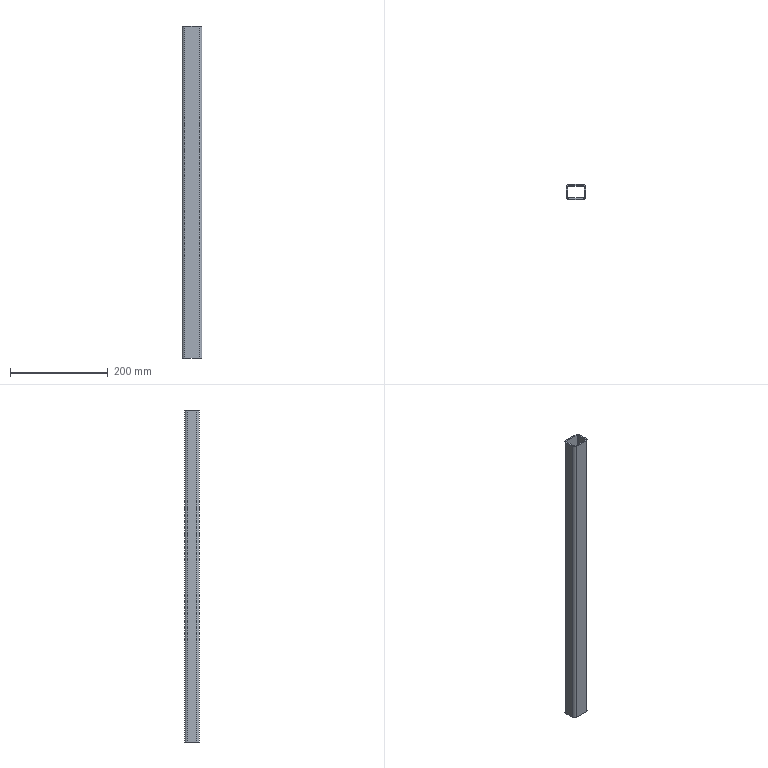Part | SolidWorks | features BaseBody 1 | 1 solid | 18 faces | box 40 x 30 x 680 mm | volume 248862 mm3 | plane 10 | cylinder 8 | commonest cylinder face diameters 4 x4 10 x4
STEP:
#1=CARTESIAN_POINT('',(17.,-10.,-340.));
#2=VERTEX_POINT('',#1);
#3=CARTESIAN_POINT('',(17.,10.,-340.));
#4=VERTEX_POINT('',#3);
#5=CARTESIAN_POINT('',(17.,10.,-340.));
#6=DIRECTION('',(0.,1.,0.));
#7=VECTOR('',#6,1000.);
#8=LINE('',#5,#7);
#9=EDGE_CURVE('',#2,#4,#8,.T.);
#10=ORIENTED_EDGE('',*,*,#9,.F.);
#11=CARTESIAN_POINT('',(17.,-10.,340.));
#12=VERTEX_POINT('',#11);
#13=CARTESIAN_POINT('',(17.,-10.,340.));
#14=DIRECTION('',(0.,0.,-1.));
#15=VECTOR('',#14,1000.);
#16=LINE('',#13,#15);
#17=EDGE_CURVE('',#12,#2,#16,.T.);
#18=ORIENTED_EDGE('',*,*,#17,.F.);
#19=CARTESIAN_POINT('',(17.,10.,340.));
#20=VERTEX_POINT('',#19);
#21=CARTESIAN_POINT('',(17.,10.,340.));
#22=DIRECTION('',(0.,1.,0.));
#23=VECTOR('',#22,1000.);
#24=LINE('',#21,#23);
#25=EDGE_CURVE('',#12,#20,#24,.T.);
#26=ORIENTED_EDGE('',*,*,#25,.T.);
#27=CARTESIAN_POINT('',(17.,10.,340.));
#28=DIRECTION('',(0.,0.,-1.));
#29=VECTOR('',#28,1000.);
#30=LINE('',#27,#29);
#31=EDGE_CURVE('',#20,#4,#30,.T.);
#32=ORIENTED_EDGE('',*,*,#31,.T.);
#33=EDGE_LOOP('',(#10,#18,#26,#32));
#34=FACE_OUTER_BOUND('',#33,.T.);
#35=CARTESIAN_POINT('',(17.,10.,340.));
#36=DIRECTION('',(-1.,0.,0.));
#37=DIRECTION('',(0.,1.,0.));
#38=AXIS2_PLACEMENT_3D('',#35,#36,#37);
#39=PLANE('',#38);
#40=ADVANCED_FACE('',(#34),#39,.T.);
#41=CARTESIAN_POINT('',(15.,-12.,-340.));
#42=VERTEX_POINT('',#41);
#43=CARTESIAN_POINT('',(15.,-10.,-340.));
#44=DIRECTION('',(0.,0.,1.));
#45=DIRECTION('',(1.,0.,0.));
#46=AXIS2_PLACEMENT_3D('',#43,#44,#45);
#47=CIRCLE('',#46,2.);
#48=EDGE_CURVE('',#42,#2,#47,.T.);
#49=ORIENTED_EDGE('',*,*,#48,.F.);
#50=CARTESIAN_POINT('',(15.,-12.,340.));
#51=VERTEX_POINT('',#50);
#52=CARTESIAN_POINT('',(15.,-12.,340.));
#53=DIRECTION('',(0.,0.,-1.));
#54=VECTOR('',#53,1000.);
#55=LINE('',#52,#54);
#56=EDGE_CURVE('',#51,#42,#55,.T.);
#57=ORIENTED_EDGE('',*,*,#56,.F.);
#58=CARTESIAN_POINT('',(15.,-10.,340.));
#59=DIRECTION('',(0.,0.,1.));
#60=DIRECTION('',(1.,0.,0.));
#61=AXIS2_PLACEMENT_3D('',#58,#59,#60);
#62=CIRCLE('',#61,2.);
#63=EDGE_CURVE('',#51,#12,#62,.T.);
#64=ORIENTED_EDGE('',*,*,#63,.T.);
#65=ORIENTED_EDGE('',*,*,#17,.T.);
#66=EDGE_LOOP('',(#49,#57,#64,#65));
#67=FACE_OUTER_BOUND('',#66,.T.);
#68=CARTESIAN_POINT('',(15.,-10.,340.));
#69=DIRECTION('',(0.,0.,-1.));
#70=DIRECTION('',(-1.,0.,0.));
#71=AXIS2_PLACEMENT_3D('',#68,#69,#70);
#72=CYLINDRICAL_SURFACE('',#71,2.);
#73=ADVANCED_FACE('',(#67),#72,.F.);
#74=CARTESIAN_POINT('',(-15.,-12.,-340.));
#75=VERTEX_POINT('',#74);
#76=CARTESIAN_POINT('',(-15.,-12.,-340.));
#77=DIRECTION('',(1.,0.,0.));
#78=VECTOR('',#77,1000.);
#79=LINE('',#76,#78);
#80=EDGE_CURVE('',#75,#42,#79,.T.);
#81=ORIENTED_EDGE('',*,*,#80,.F.);
#82=CARTESIAN_POINT('',(-15.,-12.,340.));
#83=VERTEX_POINT('',#82);
#84=CARTESIAN_POINT('',(-15.,-12.,340.));
#85=DIRECTION('',(0.,0.,-1.));
#86=VECTOR('',#85,1000.);
#87=LINE('',#84,#86);
#88=EDGE_CURVE('',#83,#75,#87,.T.);
#89=ORIENTED_EDGE('',*,*,#88,.F.);
#90=CARTESIAN_POINT('',(-15.,-12.,340.));
#91=DIRECTION('',(1.,0.,0.));
#92=VECTOR('',#91,1000.);
#93=LINE('',#90,#92);
#94=EDGE_CURVE('',#83,#51,#93,.T.);
#95=ORIENTED_EDGE('',*,*,#94,.T.);
#96=ORIENTED_EDGE('',*,*,#56,.T.);
#97=EDGE_LOOP('',(#81,#89,#95,#96));
#98=FACE_OUTER_BOUND('',#97,.T.);
#99=CARTESIAN_POINT('',(-15.,-12.,340.));
#100=DIRECTION('',(0.,1.,0.));
#101=DIRECTION('',(1.,0.,0.));
#102=AXIS2_PLACEMENT_3D('',#99,#100,#101);
#103=PLANE('',#102);
#104=ADVANCED_FACE('',(#98),#103,.T.);
#105=CARTESIAN_POINT('',(-17.,-10.,-340.));
#106=VERTEX_POINT('',#105);
#107=CARTESIAN_POINT('',(-15.,-10.,-340.));
#108=DIRECTION('',(0.,0.,1.));
#109=DIRECTION('',(1.,0.,0.));
#110=AXIS2_PLACEMENT_3D('',#107,#108,#109);
#111=CIRCLE('',#110,2.);
#112=EDGE_CURVE('',#106,#75,#111,.T.);
#113=ORIENTED_EDGE('',*,*,#112,.F.);
#114=CARTESIAN_POINT('',(-17.,-10.,340.));
#115=VERTEX_POINT('',#114);
#116=CARTESIAN_POINT('',(-17.,-10.,340.));
#117=DIRECTION('',(0.,0.,-1.));
#118=VECTOR('',#117,1000.);
#119=LINE('',#116,#118);
#120=EDGE_CURVE('',#115,#106,#119,.T.);
#121=ORIENTED_EDGE('',*,*,#120,.F.);
#122=CARTESIAN_POINT('',(-15.,-10.,340.));
#123=DIRECTION('',(0.,0.,1.));
#124=DIRECTION('',(1.,0.,0.));
#125=AXIS2_PLACEMENT_3D('',#122,#123,#124);
#126=CIRCLE('',#125,2.);
#127=EDGE_CURVE('',#115,#83,#126,.T.);
#128=ORIENTED_EDGE('',*,*,#127,.T.);
#129=ORIENTED_EDGE('',*,*,#88,.T.);
#130=EDGE_LOOP('',(#113,#121,#128,#129));
#131=FACE_OUTER_BOUND('',#130,.T.);
#132=CARTESIAN_POINT('',(-15.,-10.,340.));
#133=DIRECTION('',(0.,0.,-1.));
#134=DIRECTION('',(-1.,0.,0.));
#135=AXIS2_PLACEMENT_3D('',#132,#133,#134);
#136=CYLINDRICAL_SURFACE('',#135,2.);
#137=ADVANCED_FACE('',(#131),#136,.F.);
#138=CARTESIAN_POINT('',(-17.,10.,-340.));
#139=VERTEX_POINT('',#138);
#140=CARTESIAN_POINT('',(-17.,10.,-340.));
#141=DIRECTION('',(0.,-1.,0.));
#142=VECTOR('',#141,1000.);
#143=LINE('',#140,#142);
#144=EDGE_CURVE('',#139,#106,#143,.T.);
#145=ORIENTED_EDGE('',*,*,#144,.F.);
#146=CARTESIAN_POINT('',(-17.,10.,340.));
#147=VERTEX_POINT('',#146);
#148=CARTESIAN_POINT('',(-17.,10.,340.));
#149=DIRECTION('',(0.,0.,-1.));
#150=VECTOR('',#149,1000.);
#151=LINE('',#148,#150);
#152=EDGE_CURVE('',#147,#139,#151,.T.);
#153=ORIENTED_EDGE('',*,*,#152,.F.);
#154=CARTESIAN_POINT('',(-17.,10.,340.));
#155=DIRECTION('',(0.,-1.,0.));
#156=VECTOR('',#155,1000.);
#157=LINE('',#154,#156);
#158=EDGE_CURVE('',#147,#115,#157,.T.);
#159=ORIENTED_EDGE('',*,*,#158,.T.);
#160=ORIENTED_EDGE('',*,*,#120,.T.);
#161=EDGE_LOOP('',(#145,#153,#159,#160));
#162=FACE_OUTER_BOUND('',#161,.T.);
#163=CARTESIAN_POINT('',(-17.,10.,340.));
#164=DIRECTION('',(1.,0.,0.));
#165=DIRECTION('',(0.,1.,0.));
#166=AXIS2_PLACEMENT_3D('',#163,#164,#165);
#167=PLANE('',#166);
#168=ADVANCED_FACE('',(#162),#167,.T.);
#169=CARTESIAN_POINT('',(-15.,12.,-340.));
#170=VERTEX_POINT('',#169);
#171=CARTESIAN_POINT('',(-15.,10.,-340.));
#172=DIRECTION('',(0.,0.,1.));
#173=DIRECTION('',(1.,0.,0.));
#174=AXIS2_PLACEMENT_3D('',#171,#172,#173);
#175=CIRCLE('',#174,2.);
#176=EDGE_CURVE('',#170,#139,#175,.T.);
#177=ORIENTED_EDGE('',*,*,#176,.F.);
#178=CARTESIAN_POINT('',(-15.,12.,340.));
#179=VERTEX_POINT('',#178);
#180=CARTESIAN_POINT('',(-15.,12.,340.));
#181=DIRECTION('',(0.,0.,-1.));
#182=VECTOR('',#181,1000.);
#183=LINE('',#180,#182);
#184=EDGE_CURVE('',#179,#170,#183,.T.);
#185=ORIENTED_EDGE('',*,*,#184,.F.);
#186=CARTESIAN_POINT('',(-15.,10.,340.));
#187=DIRECTION('',(0.,0.,1.));
#188=DIRECTION('',(1.,0.,0.));
#189=AXIS2_PLACEMENT_3D('',#186,#187,#188);
#190=CIRCLE('',#189,2.);
#191=EDGE_CURVE('',#179,#147,#190,.T.);
#192=ORIENTED_EDGE('',*,*,#191,.T.);
#193=ORIENTED_EDGE('',*,*,#152,.T.);
#194=EDGE_LOOP('',(#177,#185,#192,#193));
#195=FACE_OUTER_BOUND('',#194,.T.);
#196=CARTESIAN_POINT('',(-15.,10.,340.));
#197=DIRECTION('',(0.,0.,-1.));
#198=DIRECTION('',(-1.,0.,0.));
#199=AXIS2_PLACEMENT_3D('',#196,#197,#198);
#200=CYLINDRICAL_SURFACE('',#199,2.);
#201=ADVANCED_FACE('',(#195),#200,.F.);
#202=CARTESIAN_POINT('',(15.,12.,-340.));
#203=VERTEX_POINT('',#202);
#204=CARTESIAN_POINT('',(-15.,12.,-340.));
#205=DIRECTION('',(-1.,0.,0.));
#206=VECTOR('',#205,1000.);
#207=LINE('',#204,#206);
#208=EDGE_CURVE('',#203,#170,#207,.T.);
#209=ORIENTED_EDGE('',*,*,#208,.F.);
#210=CARTESIAN_POINT('',(15.,12.,340.));
#211=VERTEX_POINT('',#210);
#212=CARTESIAN_POINT('',(15.,12.,340.));
#213=DIRECTION('',(0.,0.,-1.));
#214=VECTOR('',#213,1000.);
#215=LINE('',#212,#214);
#216=EDGE_CURVE('',#211,#203,#215,.T.);
#217=ORIENTED_EDGE('',*,*,#216,.F.);
#218=CARTESIAN_POINT('',(-15.,12.,340.));
#219=DIRECTION('',(-1.,0.,0.));
#220=VECTOR('',#219,1000.);
#221=LINE('',#218,#220);
#222=EDGE_CURVE('',#211,#179,#221,.T.);
#223=ORIENTED_EDGE('',*,*,#222,.T.);
#224=ORIENTED_EDGE('',*,*,#184,.T.);
#225=EDGE_LOOP('',(#209,#217,#223,#224));
#226=FACE_OUTER_BOUND('',#225,.T.);
#227=CARTESIAN_POINT('',(-15.,12.,340.));
#228=DIRECTION('',(0.,-1.,0.));
#229=DIRECTION('',(0.,0.,-1.));
#230=AXIS2_PLACEMENT_3D('',#227,#228,#229);
#231=PLANE('',#230);
#232=ADVANCED_FACE('',(#226),#231,.T.);
#233=CARTESIAN_POINT('',(15.,10.,-340.));
#234=DIRECTION('',(0.,0.,1.));
#235=DIRECTION('',(-1.,0.,0.));
#236=AXIS2_PLACEMENT_3D('',#233,#234,#235);
#237=CIRCLE('',#236,2.);
#238=EDGE_CURVE('',#4,#203,#237,.T.);
#239=ORIENTED_EDGE('',*,*,#238,.F.);
#240=ORIENTED_EDGE('',*,*,#31,.F.);
#241=CARTESIAN_POINT('',(15.,10.,340.));
#242=DIRECTION('',(0.,0.,1.));
#243=DIRECTION('',(-1.,0.,0.));
#244=AXIS2_PLACEMENT_3D('',#241,#242,#243);
#245=CIRCLE('',#244,2.);
#246=EDGE_CURVE('',#20,#211,#245,.T.);
#247=ORIENTED_EDGE('',*,*,#246,.T.);
#248=ORIENTED_EDGE('',*,*,#216,.T.);
#249=EDGE_LOOP('',(#239,#240,#247,#248));
#250=FACE_OUTER_BOUND('',#249,.T.);
#251=CARTESIAN_POINT('',(15.,10.,340.));
#252=DIRECTION('',(0.,0.,-1.));
#253=DIRECTION('',(-1.,0.,0.));
#254=AXIS2_PLACEMENT_3D('',#251,#252,#253);
#255=CYLINDRICAL_SURFACE('',#254,2.);
#256=ADVANCED_FACE('',(#250),#255,.F.);
#257=CARTESIAN_POINT('',(-15.,-15.,-340.));
#258=VERTEX_POINT('',#257);
#259=CARTESIAN_POINT('',(15.,-15.,-340.));
#260=VERTEX_POINT('',#259);
#261=CARTESIAN_POINT('',(-15.,-15.,-340.));
#262=DIRECTION('',(1.,0.,0.));
#263=VECTOR('',#262,1000.);
#264=LINE('',#261,#263);
#265=EDGE_CURVE('',#258,#260,#264,.T.);
#266=ORIENTED_EDGE('',*,*,#265,.T.);
#267=CARTESIAN_POINT('',(15.,-15.,340.));
#268=VERTEX_POINT('',#267);
#269=CARTESIAN_POINT('',(15.,-15.,340.));
#270=DIRECTION('',(0.,0.,-1.));
#271=VECTOR('',#270,1000.);
#272=LINE('',#269,#271);
#273=EDGE_CURVE('',#268,#260,#272,.T.);
#274=ORIENTED_EDGE('',*,*,#273,.F.);
#275=CARTESIAN_POINT('',(-15.,-15.,340.));
#276=VERTEX_POINT('',#275);
#277=CARTESIAN_POINT('',(-15.,-15.,340.));
#278=DIRECTION('',(1.,0.,0.));
#279=VECTOR('',#278,1000.);
#280=LINE('',#277,#279);
#281=EDGE_CURVE('',#276,#268,#280,.T.);
#282=ORIENTED_EDGE('',*,*,#281,.F.);
#283=CARTESIAN_POINT('',(-15.,-15.,340.));
#284=DIRECTION('',(0.,0.,-1.));
#285=VECTOR('',#284,1000.);
#286=LINE('',#283,#285);
#287=EDGE_CURVE('',#276,#258,#286,.T.);
#288=ORIENTED_EDGE('',*,*,#287,.T.);
#289=EDGE_LOOP('',(#266,#274,#282,#288));
#290=FACE_OUTER_BOUND('',#289,.T.);
#291=CARTESIAN_POINT('',(-15.,-15.,340.));
#292=DIRECTION('',(0.,1.,0.));
#293=DIRECTION('',(1.,0.,0.));
#294=AXIS2_PLACEMENT_3D('',#291,#292,#293);
#295=PLANE('',#294);
#296=ADVANCED_FACE('',(#290),#295,.F.);
#297=CARTESIAN_POINT('',(-20.,-10.,-340.));
#298=VERTEX_POINT('',#297);
#299=CARTESIAN_POINT('',(-15.,-10.,-340.));
#300=DIRECTION('',(0.,0.,1.));
#301=DIRECTION('',(1.,0.,0.));
#302=AXIS2_PLACEMENT_3D('',#299,#300,#301);
#303=CIRCLE('',#302,5.);
#304=EDGE_CURVE('',#298,#258,#303,.T.);
#305=ORIENTED_EDGE('',*,*,#304,.T.);
#306=ORIENTED_EDGE('',*,*,#287,.F.);
#307=CARTESIAN_POINT('',(-20.,-10.,340.));
#308=VERTEX_POINT('',#307);
#309=CARTESIAN_POINT('',(-15.,-10.,340.));
#310=DIRECTION('',(0.,0.,1.));
#311=DIRECTION('',(1.,0.,0.));
#312=AXIS2_PLACEMENT_3D('',#309,#310,#311);
#313=CIRCLE('',#312,5.);
#314=EDGE_CURVE('',#308,#276,#313,.T.);
#315=ORIENTED_EDGE('',*,*,#314,.F.);
#316=CARTESIAN_POINT('',(-20.,-10.,340.));
#317=DIRECTION('',(0.,0.,-1.));
#318=VECTOR('',#317,1000.);
#319=LINE('',#316,#318);
#320=EDGE_CURVE('',#308,#298,#319,.T.);
#321=ORIENTED_EDGE('',*,*,#320,.T.);
#322=EDGE_LOOP('',(#305,#306,#315,#321));
#323=FACE_OUTER_BOUND('',#322,.T.);
#324=CARTESIAN_POINT('',(-15.,-10.,340.));
#325=DIRECTION('',(0.,0.,-1.));
#326=DIRECTION('',(-1.,0.,0.));
#327=AXIS2_PLACEMENT_3D('',#324,#325,#326);
#328=CYLINDRICAL_SURFACE('',#327,5.);
#329=ADVANCED_FACE('',(#323),#328,.T.);
#330=CARTESIAN_POINT('',(-20.,10.,-340.));
#331=VERTEX_POINT('',#330);
#332=CARTESIAN_POINT('',(-20.,10.,-340.));
#333=DIRECTION('',(0.,-1.,0.));
#334=VECTOR('',#333,1000.);
#335=LINE('',#332,#334);
#336=EDGE_CURVE('',#331,#298,#335,.T.);
#337=ORIENTED_EDGE('',*,*,#336,.T.);
#338=ORIENTED_EDGE('',*,*,#320,.F.);
#339=CARTESIAN_POINT('',(-20.,10.,340.));
#340=VERTEX_POINT('',#339);
#341=CARTESIAN_POINT('',(-20.,10.,340.));
#342=DIRECTION('',(0.,-1.,0.));
#343=VECTOR('',#342,1000.);
#344=LINE('',#341,#343);
#345=EDGE_CURVE('',#340,#308,#344,.T.);
#346=ORIENTED_EDGE('',*,*,#345,.F.);
#347=CARTESIAN_POINT('',(-20.,10.,340.));
#348=DIRECTION('',(0.,0.,-1.));
#349=VECTOR('',#348,1000.);
#350=LINE('',#347,#349);
#351=EDGE_CURVE('',#340,#331,#350,.T.);
#352=ORIENTED_EDGE('',*,*,#351,.T.);
#353=EDGE_LOOP('',(#337,#338,#346,#352));
#354=FACE_OUTER_BOUND('',#353,.T.);
#355=CARTESIAN_POINT('',(-20.,10.,340.));
#356=DIRECTION('',(1.,0.,0.));
#357=DIRECTION('',(0.,-1.,0.));
#358=AXIS2_PLACEMENT_3D('',#355,#356,#357);
#359=PLANE('',#358);
#360=ADVANCED_FACE('',(#354),#359,.F.);
#361=CARTESIAN_POINT('',(-15.,15.,-340.));
#362=VERTEX_POINT('',#361);
#363=CARTESIAN_POINT('',(-15.,10.,-340.));
#364=DIRECTION('',(0.,0.,1.));
#365=DIRECTION('',(1.,0.,0.));
#366=AXIS2_PLACEMENT_3D('',#363,#364,#365);
#367=CIRCLE('',#366,5.);
#368=EDGE_CURVE('',#362,#331,#367,.T.);
#369=ORIENTED_EDGE('',*,*,#368,.T.);
#370=ORIENTED_EDGE('',*,*,#351,.F.);
#371=CARTESIAN_POINT('',(-15.,15.,340.));
#372=VERTEX_POINT('',#371);
#373=CARTESIAN_POINT('',(-15.,10.,340.));
#374=DIRECTION('',(0.,0.,1.));
#375=DIRECTION('',(1.,0.,0.));
#376=AXIS2_PLACEMENT_3D('',#373,#374,#375);
#377=CIRCLE('',#376,5.);
#378=EDGE_CURVE('',#372,#340,#377,.T.);
#379=ORIENTED_EDGE('',*,*,#378,.F.);
#380=CARTESIAN_POINT('',(-15.,15.,340.));
#381=DIRECTION('',(0.,0.,-1.));
#382=VECTOR('',#381,1000.);
#383=LINE('',#380,#382);
#384=EDGE_CURVE('',#372,#362,#383,.T.);
#385=ORIENTED_EDGE('',*,*,#384,.T.);
#386=EDGE_LOOP('',(#369,#370,#379,#385));
#387=FACE_OUTER_BOUND('',#386,.T.);
#388=CARTESIAN_POINT('',(-15.,10.,340.));
#389=DIRECTION('',(0.,0.,-1.));
#390=DIRECTION('',(-1.,0.,0.));
#391=AXIS2_PLACEMENT_3D('',#388,#389,#390);
#392=CYLINDRICAL_SURFACE('',#391,5.);
#393=ADVANCED_FACE('',(#387),#392,.T.);
#394=CARTESIAN_POINT('',(15.,15.,-340.));
#395=VERTEX_POINT('',#394);
#396=CARTESIAN_POINT('',(-15.,15.,-340.));
#397=DIRECTION('',(-1.,0.,0.));
#398=VECTOR('',#397,1000.);
#399=LINE('',#396,#398);
#400=EDGE_CURVE('',#395,#362,#399,.T.);
#401=ORIENTED_EDGE('',*,*,#400,.T.);
#402=ORIENTED_EDGE('',*,*,#384,.F.);
#403=CARTESIAN_POINT('',(15.,15.,340.));
#404=VERTEX_POINT('',#403);
#405=CARTESIAN_POINT('',(-15.,15.,340.));
#406=DIRECTION('',(-1.,0.,0.));
#407=VECTOR('',#406,1000.);
#408=LINE('',#405,#407);
#409=EDGE_CURVE('',#404,#372,#408,.T.);
#410=ORIENTED_EDGE('',*,*,#409,.F.);
#411=CARTESIAN_POINT('',(15.,15.,340.));
#412=DIRECTION('',(0.,0.,-1.));
#413=VECTOR('',#412,1000.);
#414=LINE('',#411,#413);
#415=EDGE_CURVE('',#404,#395,#414,.T.);
#416=ORIENTED_EDGE('',*,*,#415,.T.);
#417=EDGE_LOOP('',(#401,#402,#410,#416));
#418=FACE_OUTER_BOUND('',#417,.T.);
#419=CARTESIAN_POINT('',(-15.,15.,340.));
#420=DIRECTION('',(0.,-1.,0.));
#421=DIRECTION('',(0.,0.,-1.));
#422=AXIS2_PLACEMENT_3D('',#419,#420,#421);
#423=PLANE('',#422);
#424=ADVANCED_FACE('',(#418),#423,.F.);
#425=CARTESIAN_POINT('',(20.,10.,-340.));
#426=VERTEX_POINT('',#425);
#427=CARTESIAN_POINT('',(15.,10.,-340.));
#428=DIRECTION('',(0.,0.,1.));
#429=DIRECTION('',(-1.,0.,0.));
#430=AXIS2_PLACEMENT_3D('',#427,#428,#429);
#431=CIRCLE('',#430,5.);
#432=EDGE_CURVE('',#426,#395,#431,.T.);
#433=ORIENTED_EDGE('',*,*,#432,.T.);
#434=ORIENTED_EDGE('',*,*,#415,.F.);
#435=CARTESIAN_POINT('',(20.,10.,340.));
#436=VERTEX_POINT('',#435);
#437=CARTESIAN_POINT('',(15.,10.,340.));
#438=DIRECTION('',(0.,0.,1.));
#439=DIRECTION('',(-1.,0.,0.));
#440=AXIS2_PLACEMENT_3D('',#437,#438,#439);
#441=CIRCLE('',#440,5.);
#442=EDGE_CURVE('',#436,#404,#441,.T.);
#443=ORIENTED_EDGE('',*,*,#442,.F.);
#444=CARTESIAN_POINT('',(20.,10.,340.));
#445=DIRECTION('',(0.,0.,-1.));
#446=VECTOR('',#445,1000.);
#447=LINE('',#444,#446);
#448=EDGE_CURVE('',#436,#426,#447,.T.);
#449=ORIENTED_EDGE('',*,*,#448,.T.);
#450=EDGE_LOOP('',(#433,#434,#443,#449));
#451=FACE_OUTER_BOUND('',#450,.T.);
#452=CARTESIAN_POINT('',(15.,10.,340.));
#453=DIRECTION('',(0.,0.,-1.));
#454=DIRECTION('',(-1.,0.,0.));
#455=AXIS2_PLACEMENT_3D('',#452,#453,#454);
#456=CYLINDRICAL_SURFACE('',#455,5.);
#457=ADVANCED_FACE('',(#451),#456,.T.);
#458=CARTESIAN_POINT('',(20.,-10.,-340.));
#459=VERTEX_POINT('',#458);
#460=CARTESIAN_POINT('',(20.,10.,-340.));
#461=DIRECTION('',(0.,1.,0.));
#462=VECTOR('',#461,1000.);
#463=LINE('',#460,#462);
#464=EDGE_CURVE('',#459,#426,#463,.T.);
#465=ORIENTED_EDGE('',*,*,#464,.T.);
#466=ORIENTED_EDGE('',*,*,#448,.F.);
#467=CARTESIAN_POINT('',(20.,-10.,340.));
#468=VERTEX_POINT('',#467);
#469=CARTESIAN_POINT('',(20.,10.,340.));
#470=DIRECTION('',(0.,1.,0.));
#471=VECTOR('',#470,1000.);
#472=LINE('',#469,#471);
#473=EDGE_CURVE('',#468,#436,#472,.T.);
#474=ORIENTED_EDGE('',*,*,#473,.F.);
#475=CARTESIAN_POINT('',(20.,-10.,340.));
#476=DIRECTION('',(0.,0.,-1.));
#477=VECTOR('',#476,1000.);
#478=LINE('',#475,#477);
#479=EDGE_CURVE('',#468,#459,#478,.T.);
#480=ORIENTED_EDGE('',*,*,#479,.T.);
#481=EDGE_LOOP('',(#465,#466,#474,#480));
#482=FACE_OUTER_BOUND('',#481,.T.);
#483=CARTESIAN_POINT('',(20.,10.,340.));
#484=DIRECTION('',(-1.,0.,0.));
#485=DIRECTION('',(0.,1.,0.));
#486=AXIS2_PLACEMENT_3D('',#483,#484,#485);
#487=PLANE('',#486);
#488=ADVANCED_FACE('',(#482),#487,.F.);
#489=CARTESIAN_POINT('',(15.,-10.,-340.));
#490=DIRECTION('',(0.,0.,1.));
#491=DIRECTION('',(1.,0.,0.));
#492=AXIS2_PLACEMENT_3D('',#489,#490,#491);
#493=CIRCLE('',#492,5.);
#494=EDGE_CURVE('',#260,#459,#493,.T.);
#495=ORIENTED_EDGE('',*,*,#494,.T.);
#496=ORIENTED_EDGE('',*,*,#479,.F.);
#497=CARTESIAN_POINT('',(15.,-10.,340.));
#498=DIRECTION('',(0.,0.,1.));
#499=DIRECTION('',(1.,0.,0.));
#500=AXIS2_PLACEMENT_3D('',#497,#498,#499);
#501=CIRCLE('',#500,5.);
#502=EDGE_CURVE('',#268,#468,#501,.T.);
#503=ORIENTED_EDGE('',*,*,#502,.F.);
#504=ORIENTED_EDGE('',*,*,#273,.T.);
#505=EDGE_LOOP('',(#495,#496,#503,#504));
#506=FACE_OUTER_BOUND('',#505,.T.);
#507=CARTESIAN_POINT('',(15.,-10.,340.));
#508=DIRECTION('',(0.,0.,-1.));
#509=DIRECTION('',(-1.,0.,0.));
#510=AXIS2_PLACEMENT_3D('',#507,#508,#509);
#511=CYLINDRICAL_SURFACE('',#510,5.);
#512=ADVANCED_FACE('',(#506),#511,.T.);
#513=ORIENTED_EDGE('',*,*,#238,.T.);
#514=ORIENTED_EDGE('',*,*,#208,.T.);
#515=ORIENTED_EDGE('',*,*,#176,.T.);
#516=ORIENTED_EDGE('',*,*,#144,.T.);
#517=ORIENTED_EDGE('',*,*,#112,.T.);
#518=ORIENTED_EDGE('',*,*,#80,.T.);
#519=ORIENTED_EDGE('',*,*,#48,.T.);
#520=ORIENTED_EDGE('',*,*,#9,.T.);
#521=EDGE_LOOP('',(#513,#514,#515,#516,#517,#518,#519,#520));
#522=FACE_BOUND('',#521,.T.);
#523=ORIENTED_EDGE('',*,*,#494,.F.);
#524=ORIENTED_EDGE('',*,*,#265,.F.);
#525=ORIENTED_EDGE('',*,*,#304,.F.);
#526=ORIENTED_EDGE('',*,*,#336,.F.);
#527=ORIENTED_EDGE('',*,*,#368,.F.);
#528=ORIENTED_EDGE('',*,*,#400,.F.);
#529=ORIENTED_EDGE('',*,*,#432,.F.);
#530=ORIENTED_EDGE('',*,*,#464,.F.);
#531=EDGE_LOOP('',(#523,#524,#525,#526,#527,#528,#529,#530));
#532=FACE_OUTER_BOUND('',#531,.T.);
#533=CARTESIAN_POINT('',(15.,-10.,-340.));
#534=DIRECTION('',(0.,0.,1.));
#535=DIRECTION('',(1.,0.,0.));
#536=AXIS2_PLACEMENT_3D('',#533,#534,#535);
#537=PLANE('',#536);
#538=ADVANCED_FACE('',(#522,#532),#537,.F.);
#539=ORIENTED_EDGE('',*,*,#222,.F.);
#540=ORIENTED_EDGE('',*,*,#246,.F.);
#541=ORIENTED_EDGE('',*,*,#25,.F.);
#542=ORIENTED_EDGE('',*,*,#63,.F.);
#543=ORIENTED_EDGE('',*,*,#94,.F.);
#544=ORIENTED_EDGE('',*,*,#127,.F.);
#545=ORIENTED_EDGE('',*,*,#158,.F.);
#546=ORIENTED_EDGE('',*,*,#191,.F.);
#547=EDGE_LOOP('',(#539,#540,#541,#542,#543,#544,#545,#546));
#548=FACE_BOUND('',#547,.T.);
#549=ORIENTED_EDGE('',*,*,#502,.T.);
#550=ORIENTED_EDGE('',*,*,#473,.T.);
#551=ORIENTED_EDGE('',*,*,#442,.T.);
#552=ORIENTED_EDGE('',*,*,#409,.T.);
#553=ORIENTED_EDGE('',*,*,#378,.T.);
#554=ORIENTED_EDGE('',*,*,#345,.T.);
#555=ORIENTED_EDGE('',*,*,#314,.T.);
#556=ORIENTED_EDGE('',*,*,#281,.T.);
#557=EDGE_LOOP('',(#549,#550,#551,#552,#553,#554,#555,#556));
#558=FACE_OUTER_BOUND('',#557,.T.);
#559=CARTESIAN_POINT('',(15.,-10.,340.));
#560=DIRECTION('',(0.,0.,1.));
#561=DIRECTION('',(1.,0.,0.));
#562=AXIS2_PLACEMENT_3D('',#559,#560,#561);
#563=PLANE('',#562);
#564=ADVANCED_FACE('',(#548,#558),#563,.T.);
#565=CLOSED_SHELL('',(#40,#73,#104,#137,#168,#201,#232,#256,#296,#329,#360,#393,#424,#457,#488,#512,#538,#564));
#566=MANIFOLD_SOLID_BREP('',#565);
#567=CARTESIAN_POINT('',(0.,0.,0.));
#568=DIRECTION('',(0.,0.,1.));
#569=DIRECTION('',(1.,0.,0.));
#570=AXIS2_PLACEMENT_3D('',#567,#568,#569);
#571=(LENGTH_UNIT()NAMED_UNIT(*)SI_UNIT(.MILLI.,.METRE.));
#572=UNCERTAINTY_MEASURE_WITH_UNIT(LENGTH_MEASURE(0.00001),#571,'','');
#573=(NAMED_UNIT(*)PLANE_ANGLE_UNIT()SI_UNIT($,.RADIAN.));
#574=(NAMED_UNIT(*)SI_UNIT($,.STERADIAN.)SOLID_ANGLE_UNIT());
#575=(GEOMETRIC_REPRESENTATION_CONTEXT(3)GLOBAL_UNCERTAINTY_ASSIGNED_CONTEXT((#572))GLOBAL_UNIT_ASSIGNED_CONTEXT((#571,#573,#574))REPRESENTATION_CONTEXT('',''));
#576=ADVANCED_BREP_SHAPE_REPRESENTATION('',(#566,#570),#575);